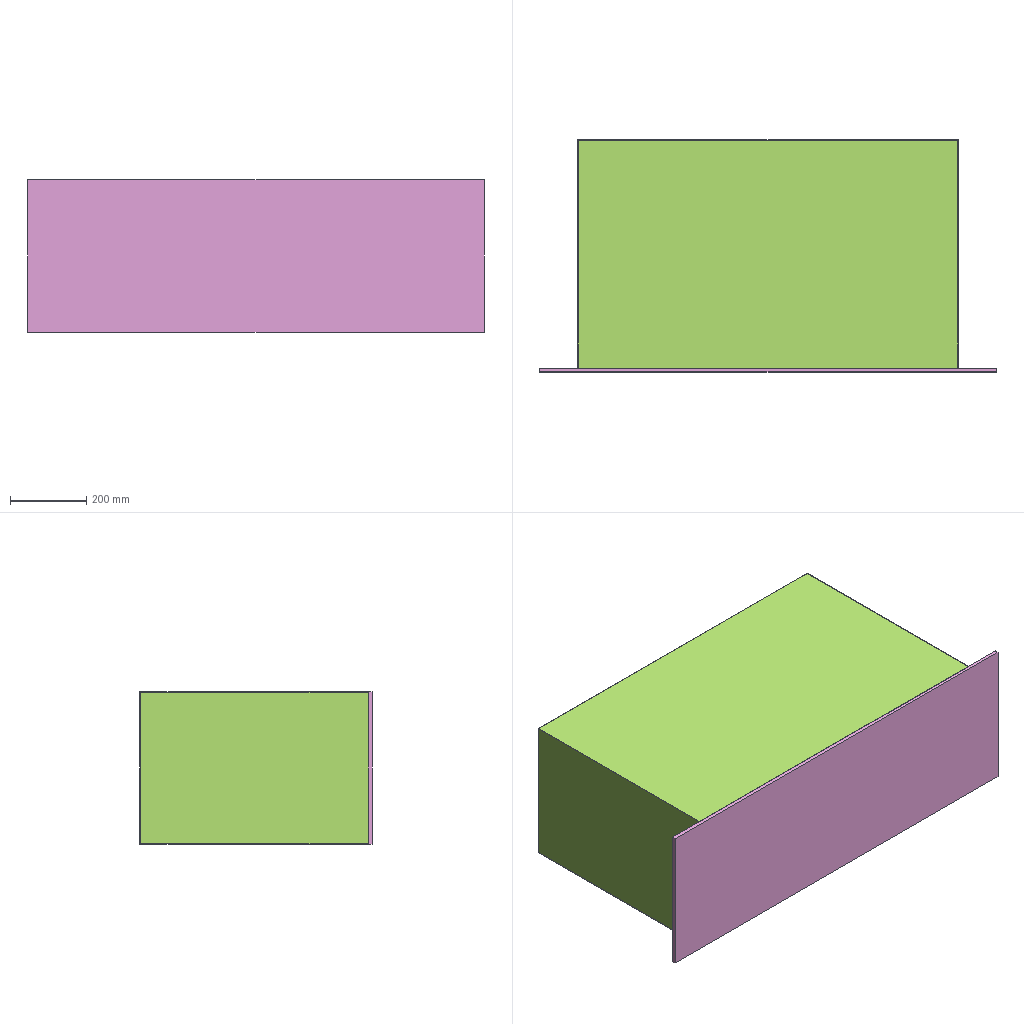Assembly | SolidWorks | 8 different items | 10 placed | box 1200 x 610 x 400 mm
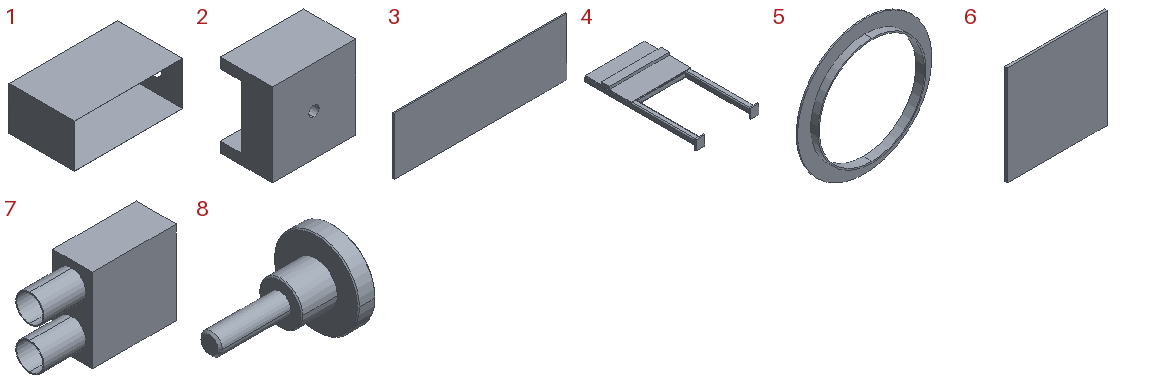Parts list (item | quantity | size | volume | features):
1 | x1 | 1000 x 600 x 400 mm | 2057133 mm3 | features Cut 1, Extrusion 1, ICE 1
2 | x2 | 40 x 25 x 40 mm | 27705 mm3 | features Extrusion 1, HoleWzd 1, ICE 1
3 | x1 | 1200 x 10 x 400 mm | 4800000 mm3 | features Extrusion 1
4 | x1 | 231.174 x 415 x 40.019 mm | 315048 mm3 | features ICE 3, WeldMemberFeat 1, WeldmentFeature 1
5 | x1 | 186 x 12 x 186 mm | 30159 mm3 | features Extrusion 1, ICE 1
6 | x1 | 80 x 2 x 80 mm | 12800 mm3 | features Extrusion 1
7 | x1 | 120 x 38 x 80 mm | 39835 mm3 | features ICE 2, Cut 1, Extrusion 1
8 | x2 | 35.1 x 24 x 24 mm | 3977 mm3 | features BaseBody 1
Mates (type | each side: item.copy, entity, surface, feature):
Coincident | 7.1 edge | 6.1 edge
Coincident | 7.1 face plane Boss-Extrude1 | 6.1 face plane Boss-Extrude1
Coincident | 3.1 plane | assembly plane | 3 times
Coincident | 1.1 face plane Boss-Extrude1 | 3.1 face plane Boss-Extrude1 | 2 times
Width | 1.1 face plane Boss-Extrude1 | 1.1 face plane Boss-Extrude1 | 3.1 face plane Boss-Extrude1 | 3.1 face plane Boss-Extrude1
Concentric | 1.1 edge | 5.1 face cylinder Boss-Extrude1
Coincident | 1.1 face plane Boss-Extrude1 | 5.1 face plane Boss-Extrude2
Parallel | 7.1 face plane Boss-Extrude1 | 3.1 face plane Boss-Extrude1
Coincident | 3.1 face plane Boss-Extrude1 | 4.1 face plane Boss-Extrude1
Width | 7.1 face plane Boss-Extrude1 | 7.1 face plane Boss-Extrude1 | 4.1 face plane GB/6728-1986 square hollow section 020 X 20 X 1.75(1) | 4.1 face plane GB/6728-1986 square hollow section 020 X 20 X 1.75(1) | 2 times
Coincident | 4.1 face plane Boss-Extrude3 | 2.1 face plane Cut-Extrude1 | 2 times
Coincident | 2.1 face plane Boss-Extrude1 | 2.2 face plane Boss-Extrude1 | 2 times
Concentric | 2.1 face cylinder M6 Tapped Hole1 | 8.1 face cylinder Input1
Coincident | 4.1 face plane Boss-Extrude3 | 8.1 face plane Input1
Concentric | 2.2 face cylinder M6 Tapped Hole1 | 8.2 face cylinder Input1
Coincident | 8.1 face plane Input1 | 8.2 face plane Input1
Coincident | 7.1 face plane Boss-Extrude1 | 4.1 face plane Boss-Extrude3
Coincident | 7.1 face plane Boss-Extrude1 | 2.1 face plane Boss-Extrude1
Coincident | 7.1 face plane Boss-Extrude1 | 2.2 face plane Boss-Extrude1
DistanceDim | 7.1 face plane Boss-Extrude1 | 2.1 face plane Boss-Extrude1
Parallel | 1.1 face plane Boss-Extrude1 | 4.1 face plane Boss-Extrude2